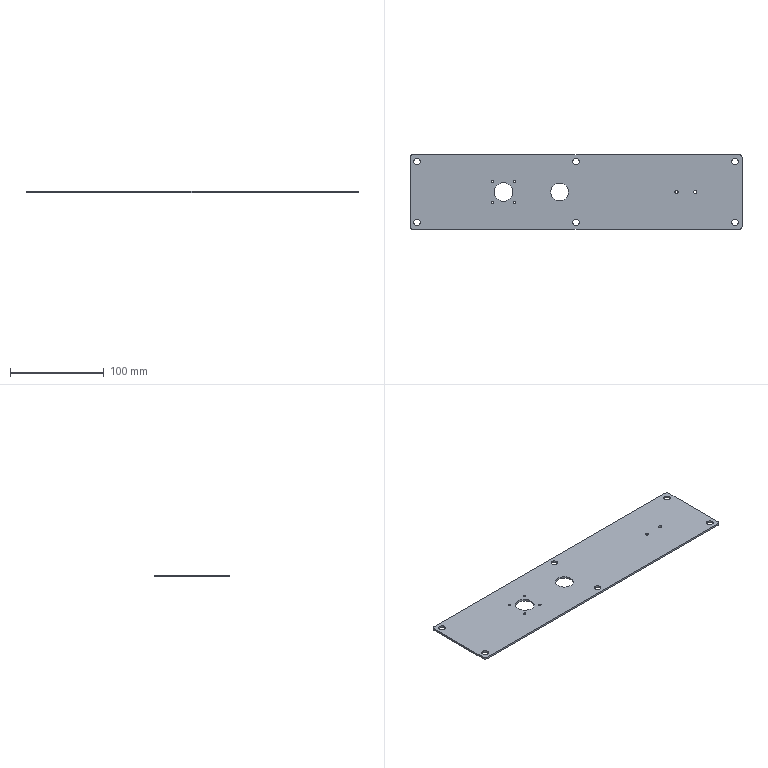Part | NX | features solid 2 | 1 solid | 38 faces | box 355 x 80 x 2 mm | volume 55052 mm3 | cylinder 32 | plane 6 | commonest cylinder face diameters 7 x12 2.459 x8 3.459 x4 6 x4 19 x2 20 x2
STEP:
#1=CARTESIAN_POINT('',(-469.229,-1630.,298.));
#2=VERTEX_POINT('',#1);
#3=CARTESIAN_POINT('',(-469.229,-1630.,300.));
#4=VERTEX_POINT('',#3);
#5=CARTESIAN_POINT('',(-469.229,-1630.,661.908));
#6=DIRECTION('',(0.,0.,-1.));
#7=VECTOR('',#6,1000.);
#8=LINE('',#5,#7);
#9=EDGE_CURVE('',#2,#4,#8,.F.);
#10=ORIENTED_EDGE('',*,*,#9,.T.);
#11=CARTESIAN_POINT('',(-465.771,-1630.,300.));
#12=VERTEX_POINT('',#11);
#13=CARTESIAN_POINT('',(-467.5,-1630.,300.));
#14=DIRECTION('',(0.,0.,1.));
#15=DIRECTION('',(-1.,0.,0.));
#16=AXIS2_PLACEMENT_3D('',#13,#14,#15);
#17=CIRCLE('',#16,1.73);
#18=EDGE_CURVE('',#4,#12,#17,.T.);
#19=ORIENTED_EDGE('',*,*,#18,.T.);
#20=CARTESIAN_POINT('',(-465.771,-1630.,298.));
#21=VERTEX_POINT('',#20);
#22=CARTESIAN_POINT('',(-465.771,-1630.,661.908));
#23=DIRECTION('',(0.,0.,-1.));
#24=VECTOR('',#23,1000.);
#25=LINE('',#22,#24);
#26=EDGE_CURVE('',#12,#21,#25,.T.);
#27=ORIENTED_EDGE('',*,*,#26,.T.);
#28=CARTESIAN_POINT('',(-467.5,-1630.,298.));
#29=DIRECTION('',(0.,0.,-1.));
#30=DIRECTION('',(1.,0.,0.));
#31=AXIS2_PLACEMENT_3D('',#28,#29,#30);
#32=CIRCLE('',#31,1.73);
#33=EDGE_CURVE('',#21,#2,#32,.T.);
#34=ORIENTED_EDGE('',*,*,#33,.T.);
#35=EDGE_LOOP('',(#10,#19,#27,#34));
#36=FACE_BOUND('',#35,.T.);
#37=CARTESIAN_POINT('',(-467.5,-1630.,661.908));
#38=DIRECTION('',(0.,0.,-1.));
#39=DIRECTION('',(1.,0.,0.));
#40=AXIS2_PLACEMENT_3D('',#37,#38,#39);
#41=CYLINDRICAL_SURFACE('',#40,1.73);
#42=ADVANCED_FACE('',(#36),#41,.F.);
#43=CARTESIAN_POINT('',(-489.229,-1630.,300.));
#44=VERTEX_POINT('',#43);
#45=CARTESIAN_POINT('',(-489.229,-1630.,298.));
#46=VERTEX_POINT('',#45);
#47=CARTESIAN_POINT('',(-489.229,-1630.,661.908));
#48=DIRECTION('',(0.,0.,-1.));
#49=VECTOR('',#48,1000.);
#50=LINE('',#47,#49);
#51=EDGE_CURVE('',#44,#46,#50,.T.);
#52=ORIENTED_EDGE('',*,*,#51,.F.);
#53=CARTESIAN_POINT('',(-485.771,-1630.,300.));
#54=VERTEX_POINT('',#53);
#55=CARTESIAN_POINT('',(-487.5,-1630.,300.));
#56=DIRECTION('',(0.,0.,1.));
#57=DIRECTION('',(-1.,0.,0.));
#58=AXIS2_PLACEMENT_3D('',#55,#56,#57);
#59=CIRCLE('',#58,1.73);
#60=EDGE_CURVE('',#44,#54,#59,.T.);
#61=ORIENTED_EDGE('',*,*,#60,.T.);
#62=CARTESIAN_POINT('',(-485.771,-1630.,298.));
#63=VERTEX_POINT('',#62);
#64=CARTESIAN_POINT('',(-485.771,-1630.,661.908));
#65=DIRECTION('',(0.,0.,-1.));
#66=VECTOR('',#65,1000.);
#67=LINE('',#64,#66);
#68=EDGE_CURVE('',#63,#54,#67,.F.);
#69=ORIENTED_EDGE('',*,*,#68,.F.);
#70=CARTESIAN_POINT('',(-487.5,-1630.,298.));
#71=DIRECTION('',(0.,0.,-1.));
#72=DIRECTION('',(1.,0.,0.));
#73=AXIS2_PLACEMENT_3D('',#70,#71,#72);
#74=CIRCLE('',#73,1.73);
#75=EDGE_CURVE('',#63,#46,#74,.T.);
#76=ORIENTED_EDGE('',*,*,#75,.T.);
#77=EDGE_LOOP('',(#52,#61,#69,#76));
#78=FACE_BOUND('',#77,.T.);
#79=CARTESIAN_POINT('',(-487.5,-1630.,661.908));
#80=DIRECTION('',(0.,0.,-1.));
#81=DIRECTION('',(1.,0.,0.));
#82=AXIS2_PLACEMENT_3D('',#79,#80,#81);
#83=CYLINDRICAL_SURFACE('',#82,1.73);
#84=ADVANCED_FACE('',(#78),#83,.F.);
#85=CARTESIAN_POINT('',(-659.78,-1641.49,300.));
#86=VERTEX_POINT('',#85);
#87=CARTESIAN_POINT('',(-659.78,-1641.49,298.));
#88=VERTEX_POINT('',#87);
#89=CARTESIAN_POINT('',(-659.78,-1641.49,-63.908));
#90=DIRECTION('',(0.,0.,1.));
#91=VECTOR('',#90,1000.);
#92=LINE('',#89,#91);
#93=EDGE_CURVE('',#86,#88,#92,.F.);
#94=ORIENTED_EDGE('',*,*,#93,.T.);
#95=CARTESIAN_POINT('',(-662.239,-1641.49,298.));
#96=VERTEX_POINT('',#95);
#97=CARTESIAN_POINT('',(-661.01,-1641.49,298.));
#98=DIRECTION('',(0.,0.,1.));
#99=DIRECTION('',(-1.,0.,0.));
#100=AXIS2_PLACEMENT_3D('',#97,#98,#99);
#101=CIRCLE('',#100,1.23);
#102=EDGE_CURVE('',#96,#88,#101,.T.);
#103=ORIENTED_EDGE('',*,*,#102,.F.);
#104=CARTESIAN_POINT('',(-662.239,-1641.49,300.));
#105=VERTEX_POINT('',#104);
#106=CARTESIAN_POINT('',(-662.239,-1641.49,-63.908));
#107=DIRECTION('',(0.,0.,1.));
#108=VECTOR('',#107,1000.);
#109=LINE('',#106,#108);
#110=EDGE_CURVE('',#96,#105,#109,.T.);
#111=ORIENTED_EDGE('',*,*,#110,.T.);
#112=CARTESIAN_POINT('',(-661.01,-1641.49,300.));
#113=DIRECTION('',(0.,0.,1.));
#114=DIRECTION('',(-1.,0.,0.));
#115=AXIS2_PLACEMENT_3D('',#112,#113,#114);
#116=CIRCLE('',#115,1.23);
#117=EDGE_CURVE('',#105,#86,#116,.T.);
#118=ORIENTED_EDGE('',*,*,#117,.T.);
#119=EDGE_LOOP('',(#94,#103,#111,#118));
#120=FACE_BOUND('',#119,.T.);
#121=CARTESIAN_POINT('',(-661.01,-1641.49,-63.908));
#122=DIRECTION('',(0.,0.,1.));
#123=DIRECTION('',(-1.,0.,0.));
#124=AXIS2_PLACEMENT_3D('',#121,#122,#123);
#125=CYLINDRICAL_SURFACE('',#124,1.23);
#126=ADVANCED_FACE('',(#120),#125,.F.);
#127=CARTESIAN_POINT('',(-659.78,-1618.51,298.));
#128=VERTEX_POINT('',#127);
#129=CARTESIAN_POINT('',(-659.78,-1618.51,300.));
#130=VERTEX_POINT('',#129);
#131=CARTESIAN_POINT('',(-659.78,-1618.51,-63.908));
#132=DIRECTION('',(0.,0.,1.));
#133=VECTOR('',#132,1000.);
#134=LINE('',#131,#133);
#135=EDGE_CURVE('',#128,#130,#134,.T.);
#136=ORIENTED_EDGE('',*,*,#135,.F.);
#137=CARTESIAN_POINT('',(-662.239,-1618.51,298.));
#138=VERTEX_POINT('',#137);
#139=CARTESIAN_POINT('',(-661.01,-1618.51,298.));
#140=DIRECTION('',(0.,0.,1.));
#141=DIRECTION('',(-1.,0.,0.));
#142=AXIS2_PLACEMENT_3D('',#139,#140,#141);
#143=CIRCLE('',#142,1.23);
#144=EDGE_CURVE('',#138,#128,#143,.T.);
#145=ORIENTED_EDGE('',*,*,#144,.F.);
#146=CARTESIAN_POINT('',(-662.239,-1618.51,300.));
#147=VERTEX_POINT('',#146);
#148=CARTESIAN_POINT('',(-662.239,-1618.51,-63.908));
#149=DIRECTION('',(0.,0.,1.));
#150=VECTOR('',#149,1000.);
#151=LINE('',#148,#150);
#152=EDGE_CURVE('',#147,#138,#151,.F.);
#153=ORIENTED_EDGE('',*,*,#152,.F.);
#154=CARTESIAN_POINT('',(-661.01,-1618.51,300.));
#155=DIRECTION('',(0.,0.,1.));
#156=DIRECTION('',(-1.,0.,0.));
#157=AXIS2_PLACEMENT_3D('',#154,#155,#156);
#158=CIRCLE('',#157,1.23);
#159=EDGE_CURVE('',#147,#130,#158,.T.);
#160=ORIENTED_EDGE('',*,*,#159,.T.);
#161=EDGE_LOOP('',(#136,#145,#153,#160));
#162=FACE_BOUND('',#161,.T.);
#163=CARTESIAN_POINT('',(-661.01,-1618.51,-63.908));
#164=DIRECTION('',(0.,0.,1.));
#165=DIRECTION('',(-1.,0.,0.));
#166=AXIS2_PLACEMENT_3D('',#163,#164,#165);
#167=CYLINDRICAL_SURFACE('',#166,1.23);
#168=ADVANCED_FACE('',(#162),#167,.F.);
#169=CARTESIAN_POINT('',(-682.761,-1618.51,300.));
#170=VERTEX_POINT('',#169);
#171=CARTESIAN_POINT('',(-682.761,-1618.51,298.));
#172=VERTEX_POINT('',#171);
#173=CARTESIAN_POINT('',(-682.761,-1618.51,-63.908));
#174=DIRECTION('',(0.,0.,1.));
#175=VECTOR('',#174,1000.);
#176=LINE('',#173,#175);
#177=EDGE_CURVE('',#170,#172,#176,.F.);
#178=ORIENTED_EDGE('',*,*,#177,.T.);
#179=CARTESIAN_POINT('',(-685.22,-1618.51,298.));
#180=VERTEX_POINT('',#179);
#181=CARTESIAN_POINT('',(-683.99,-1618.51,298.));
#182=DIRECTION('',(0.,0.,1.));
#183=DIRECTION('',(-1.,0.,0.));
#184=AXIS2_PLACEMENT_3D('',#181,#182,#183);
#185=CIRCLE('',#184,1.23);
#186=EDGE_CURVE('',#180,#172,#185,.T.);
#187=ORIENTED_EDGE('',*,*,#186,.F.);
#188=CARTESIAN_POINT('',(-685.22,-1618.51,300.));
#189=VERTEX_POINT('',#188);
#190=CARTESIAN_POINT('',(-685.22,-1618.51,-63.908));
#191=DIRECTION('',(0.,0.,1.));
#192=VECTOR('',#191,1000.);
#193=LINE('',#190,#192);
#194=EDGE_CURVE('',#180,#189,#193,.T.);
#195=ORIENTED_EDGE('',*,*,#194,.T.);
#196=CARTESIAN_POINT('',(-683.99,-1618.51,300.));
#197=DIRECTION('',(0.,0.,1.));
#198=DIRECTION('',(-1.,0.,0.));
#199=AXIS2_PLACEMENT_3D('',#196,#197,#198);
#200=CIRCLE('',#199,1.23);
#201=EDGE_CURVE('',#189,#170,#200,.T.);
#202=ORIENTED_EDGE('',*,*,#201,.T.);
#203=EDGE_LOOP('',(#178,#187,#195,#202));
#204=FACE_BOUND('',#203,.T.);
#205=CARTESIAN_POINT('',(-683.99,-1618.51,-63.908));
#206=DIRECTION('',(0.,0.,1.));
#207=DIRECTION('',(-1.,0.,0.));
#208=AXIS2_PLACEMENT_3D('',#205,#206,#207);
#209=CYLINDRICAL_SURFACE('',#208,1.23);
#210=ADVANCED_FACE('',(#204),#209,.F.);
#211=CARTESIAN_POINT('',(-682.761,-1641.49,300.));
#212=VERTEX_POINT('',#211);
#213=CARTESIAN_POINT('',(-682.761,-1641.49,298.));
#214=VERTEX_POINT('',#213);
#215=CARTESIAN_POINT('',(-682.761,-1641.49,-63.908));
#216=DIRECTION('',(0.,0.,1.));
#217=VECTOR('',#216,1000.);
#218=LINE('',#215,#217);
#219=EDGE_CURVE('',#212,#214,#218,.F.);
#220=ORIENTED_EDGE('',*,*,#219,.T.);
#221=CARTESIAN_POINT('',(-685.22,-1641.49,298.));
#222=VERTEX_POINT('',#221);
#223=CARTESIAN_POINT('',(-683.99,-1641.49,298.));
#224=DIRECTION('',(0.,0.,1.));
#225=DIRECTION('',(-1.,0.,0.));
#226=AXIS2_PLACEMENT_3D('',#223,#224,#225);
#227=CIRCLE('',#226,1.23);
#228=EDGE_CURVE('',#222,#214,#227,.T.);
#229=ORIENTED_EDGE('',*,*,#228,.F.);
#230=CARTESIAN_POINT('',(-685.22,-1641.49,300.));
#231=VERTEX_POINT('',#230);
#232=CARTESIAN_POINT('',(-685.22,-1641.49,-63.908));
#233=DIRECTION('',(0.,0.,1.));
#234=VECTOR('',#233,1000.);
#235=LINE('',#232,#234);
#236=EDGE_CURVE('',#222,#231,#235,.T.);
#237=ORIENTED_EDGE('',*,*,#236,.T.);
#238=CARTESIAN_POINT('',(-683.99,-1641.49,300.));
#239=DIRECTION('',(0.,0.,1.));
#240=DIRECTION('',(-1.,0.,0.));
#241=AXIS2_PLACEMENT_3D('',#238,#239,#240);
#242=CIRCLE('',#241,1.23);
#243=EDGE_CURVE('',#231,#212,#242,.T.);
#244=ORIENTED_EDGE('',*,*,#243,.T.);
#245=EDGE_LOOP('',(#220,#229,#237,#244));
#246=FACE_BOUND('',#245,.T.);
#247=CARTESIAN_POINT('',(-683.99,-1641.49,-63.908));
#248=DIRECTION('',(0.,0.,1.));
#249=DIRECTION('',(-1.,0.,0.));
#250=AXIS2_PLACEMENT_3D('',#247,#248,#249);
#251=CYLINDRICAL_SURFACE('',#250,1.23);
#252=ADVANCED_FACE('',(#246),#251,.F.);
#253=CARTESIAN_POINT('',(-598.5,-1662.5,298.));
#254=VERTEX_POINT('',#253);
#255=CARTESIAN_POINT('',(-598.5,-1662.5,300.));
#256=VERTEX_POINT('',#255);
#257=CARTESIAN_POINT('',(-598.5,-1662.5,298.));
#258=DIRECTION('',(0.,0.,1.));
#259=VECTOR('',#258,1000.);
#260=LINE('',#257,#259);
#261=EDGE_CURVE('',#254,#256,#260,.T.);
#262=ORIENTED_EDGE('',*,*,#261,.F.);
#263=CARTESIAN_POINT('',(-591.5,-1662.5,298.));
#264=VERTEX_POINT('',#263);
#265=CARTESIAN_POINT('',(-595.,-1662.5,298.));
#266=DIRECTION('',(0.,0.,1.));
#267=DIRECTION('',(1.,0.,0.));
#268=AXIS2_PLACEMENT_3D('',#265,#266,#267);
#269=CIRCLE('',#268,3.5);
#270=EDGE_CURVE('',#264,#254,#269,.T.);
#271=ORIENTED_EDGE('',*,*,#270,.F.);
#272=CARTESIAN_POINT('',(-591.5,-1662.5,300.));
#273=VERTEX_POINT('',#272);
#274=CARTESIAN_POINT('',(-591.5,-1662.5,298.));
#275=DIRECTION('',(0.,0.,1.));
#276=VECTOR('',#275,1000.);
#277=LINE('',#274,#276);
#278=EDGE_CURVE('',#273,#264,#277,.F.);
#279=ORIENTED_EDGE('',*,*,#278,.F.);
#280=CARTESIAN_POINT('',(-595.,-1662.5,300.));
#281=DIRECTION('',(0.,0.,-1.));
#282=DIRECTION('',(1.,0.,0.));
#283=AXIS2_PLACEMENT_3D('',#280,#281,#282);
#284=CIRCLE('',#283,3.5);
#285=EDGE_CURVE('',#256,#273,#284,.T.);
#286=ORIENTED_EDGE('',*,*,#285,.F.);
#287=EDGE_LOOP('',(#262,#271,#279,#286));
#288=FACE_BOUND('',#287,.T.);
#289=CARTESIAN_POINT('',(-595.,-1662.5,298.));
#290=DIRECTION('',(0.,0.,1.));
#291=DIRECTION('',(1.,0.,0.));
#292=AXIS2_PLACEMENT_3D('',#289,#290,#291);
#293=CYLINDRICAL_SURFACE('',#292,3.5);
#294=ADVANCED_FACE('',(#288),#293,.F.);
#295=CARTESIAN_POINT('',(-598.5,-1597.5,300.));
#296=VERTEX_POINT('',#295);
#297=CARTESIAN_POINT('',(-598.5,-1597.5,298.));
#298=VERTEX_POINT('',#297);
#299=CARTESIAN_POINT('',(-598.5,-1597.5,298.));
#300=DIRECTION('',(0.,0.,1.));
#301=VECTOR('',#300,1000.);
#302=LINE('',#299,#301);
#303=EDGE_CURVE('',#296,#298,#302,.F.);
#304=ORIENTED_EDGE('',*,*,#303,.T.);
#305=CARTESIAN_POINT('',(-591.5,-1597.5,298.));
#306=VERTEX_POINT('',#305);
#307=CARTESIAN_POINT('',(-595.,-1597.5,298.));
#308=DIRECTION('',(0.,0.,1.));
#309=DIRECTION('',(1.,0.,0.));
#310=AXIS2_PLACEMENT_3D('',#307,#308,#309);
#311=CIRCLE('',#310,3.5);
#312=EDGE_CURVE('',#306,#298,#311,.T.);
#313=ORIENTED_EDGE('',*,*,#312,.F.);
#314=CARTESIAN_POINT('',(-591.5,-1597.5,300.));
#315=VERTEX_POINT('',#314);
#316=CARTESIAN_POINT('',(-591.5,-1597.5,298.));
#317=DIRECTION('',(0.,0.,1.));
#318=VECTOR('',#317,1000.);
#319=LINE('',#316,#318);
#320=EDGE_CURVE('',#306,#315,#319,.T.);
#321=ORIENTED_EDGE('',*,*,#320,.T.);
#322=CARTESIAN_POINT('',(-595.,-1597.5,300.));
#323=DIRECTION('',(0.,0.,-1.));
#324=DIRECTION('',(1.,0.,0.));
#325=AXIS2_PLACEMENT_3D('',#322,#323,#324);
#326=CIRCLE('',#325,3.5);
#327=EDGE_CURVE('',#296,#315,#326,.T.);
#328=ORIENTED_EDGE('',*,*,#327,.F.);
#329=EDGE_LOOP('',(#304,#313,#321,#328));
#330=FACE_BOUND('',#329,.T.);
#331=CARTESIAN_POINT('',(-595.,-1597.5,298.));
#332=DIRECTION('',(0.,0.,1.));
#333=DIRECTION('',(1.,0.,0.));
#334=AXIS2_PLACEMENT_3D('',#331,#332,#333);
#335=CYLINDRICAL_SURFACE('',#334,3.5);
#336=ADVANCED_FACE('',(#330),#335,.F.);
#337=CARTESIAN_POINT('',(-768.5,-1597.5,300.));
#338=VERTEX_POINT('',#337);
#339=CARTESIAN_POINT('',(-768.5,-1597.5,298.));
#340=VERTEX_POINT('',#339);
#341=CARTESIAN_POINT('',(-768.5,-1597.5,298.));
#342=DIRECTION('',(0.,0.,1.));
#343=VECTOR('',#342,1000.);
#344=LINE('',#341,#343);
#345=EDGE_CURVE('',#338,#340,#344,.F.);
#346=ORIENTED_EDGE('',*,*,#345,.T.);
#347=CARTESIAN_POINT('',(-761.5,-1597.5,298.));
#348=VERTEX_POINT('',#347);
#349=CARTESIAN_POINT('',(-765.,-1597.5,298.));
#350=DIRECTION('',(0.,0.,1.));
#351=DIRECTION('',(1.,0.,0.));
#352=AXIS2_PLACEMENT_3D('',#349,#350,#351);
#353=CIRCLE('',#352,3.5);
#354=EDGE_CURVE('',#348,#340,#353,.T.);
#355=ORIENTED_EDGE('',*,*,#354,.F.);
#356=CARTESIAN_POINT('',(-761.5,-1597.5,300.));
#357=VERTEX_POINT('',#356);
#358=CARTESIAN_POINT('',(-761.5,-1597.5,298.));
#359=DIRECTION('',(0.,0.,1.));
#360=VECTOR('',#359,1000.);
#361=LINE('',#358,#360);
#362=EDGE_CURVE('',#348,#357,#361,.T.);
#363=ORIENTED_EDGE('',*,*,#362,.T.);
#364=CARTESIAN_POINT('',(-765.,-1597.5,300.));
#365=DIRECTION('',(0.,0.,-1.));
#366=DIRECTION('',(1.,0.,0.));
#367=AXIS2_PLACEMENT_3D('',#364,#365,#366);
#368=CIRCLE('',#367,3.5);
#369=EDGE_CURVE('',#338,#357,#368,.T.);
#370=ORIENTED_EDGE('',*,*,#369,.F.);
#371=EDGE_LOOP('',(#346,#355,#363,#370));
#372=FACE_BOUND('',#371,.T.);
#373=CARTESIAN_POINT('',(-765.,-1597.5,298.));
#374=DIRECTION('',(0.,0.,1.));
#375=DIRECTION('',(1.,0.,0.));
#376=AXIS2_PLACEMENT_3D('',#373,#374,#375);
#377=CYLINDRICAL_SURFACE('',#376,3.5);
#378=ADVANCED_FACE('',(#372),#377,.F.);
#379=CARTESIAN_POINT('',(-428.5,-1597.5,300.));
#380=VERTEX_POINT('',#379);
#381=CARTESIAN_POINT('',(-428.5,-1597.5,298.));
#382=VERTEX_POINT('',#381);
#383=CARTESIAN_POINT('',(-428.5,-1597.5,298.));
#384=DIRECTION('',(0.,0.,1.));
#385=VECTOR('',#384,1000.);
#386=LINE('',#383,#385);
#387=EDGE_CURVE('',#380,#382,#386,.F.);
#388=ORIENTED_EDGE('',*,*,#387,.T.);
#389=CARTESIAN_POINT('',(-421.5,-1597.5,298.));
#390=VERTEX_POINT('',#389);
#391=CARTESIAN_POINT('',(-425.,-1597.5,298.));
#392=DIRECTION('',(0.,0.,1.));
#393=DIRECTION('',(1.,0.,0.));
#394=AXIS2_PLACEMENT_3D('',#391,#392,#393);
#395=CIRCLE('',#394,3.5);
#396=EDGE_CURVE('',#390,#382,#395,.T.);
#397=ORIENTED_EDGE('',*,*,#396,.F.);
#398=CARTESIAN_POINT('',(-421.5,-1597.5,300.));
#399=VERTEX_POINT('',#398);
#400=CARTESIAN_POINT('',(-421.5,-1597.5,298.));
#401=DIRECTION('',(0.,0.,1.));
#402=VECTOR('',#401,1000.);
#403=LINE('',#400,#402);
#404=EDGE_CURVE('',#390,#399,#403,.T.);
#405=ORIENTED_EDGE('',*,*,#404,.T.);
#406=CARTESIAN_POINT('',(-425.,-1597.5,300.));
#407=DIRECTION('',(0.,0.,-1.));
#408=DIRECTION('',(1.,0.,0.));
#409=AXIS2_PLACEMENT_3D('',#406,#407,#408);
#410=CIRCLE('',#409,3.5);
#411=EDGE_CURVE('',#380,#399,#410,.T.);
#412=ORIENTED_EDGE('',*,*,#411,.F.);
#413=EDGE_LOOP('',(#388,#397,#405,#412));
#414=FACE_BOUND('',#413,.T.);
#415=CARTESIAN_POINT('',(-425.,-1597.5,298.));
#416=DIRECTION('',(0.,0.,1.));
#417=DIRECTION('',(1.,0.,0.));
#418=AXIS2_PLACEMENT_3D('',#415,#416,#417);
#419=CYLINDRICAL_SURFACE('',#418,3.5);
#420=ADVANCED_FACE('',(#414),#419,.F.);
#421=CARTESIAN_POINT('',(-428.5,-1662.5,300.));
#422=VERTEX_POINT('',#421);
#423=CARTESIAN_POINT('',(-428.5,-1662.5,298.));
#424=VERTEX_POINT('',#423);
#425=CARTESIAN_POINT('',(-428.5,-1662.5,298.));
#426=DIRECTION('',(0.,0.,1.));
#427=VECTOR('',#426,1000.);
#428=LINE('',#425,#427);
#429=EDGE_CURVE('',#422,#424,#428,.F.);
#430=ORIENTED_EDGE('',*,*,#429,.T.);
#431=CARTESIAN_POINT('',(-421.5,-1662.5,298.));
#432=VERTEX_POINT('',#431);
#433=CARTESIAN_POINT('',(-425.,-1662.5,298.));
#434=DIRECTION('',(0.,0.,1.));
#435=DIRECTION('',(1.,0.,0.));
#436=AXIS2_PLACEMENT_3D('',#433,#434,#435);
#437=CIRCLE('',#436,3.5);
#438=EDGE_CURVE('',#432,#424,#437,.T.);
#439=ORIENTED_EDGE('',*,*,#438,.F.);
#440=CARTESIAN_POINT('',(-421.5,-1662.5,300.));
#441=VERTEX_POINT('',#440);
#442=CARTESIAN_POINT('',(-421.5,-1662.5,298.));
#443=DIRECTION('',(0.,0.,1.));
#444=VECTOR('',#443,1000.);
#445=LINE('',#442,#444);
#446=EDGE_CURVE('',#432,#441,#445,.T.);
#447=ORIENTED_EDGE('',*,*,#446,.T.);
#448=CARTESIAN_POINT('',(-425.,-1662.5,300.));
#449=DIRECTION('',(0.,0.,-1.));
#450=DIRECTION('',(1.,0.,0.));
#451=AXIS2_PLACEMENT_3D('',#448,#449,#450);
#452=CIRCLE('',#451,3.5);
#453=EDGE_CURVE('',#422,#441,#452,.T.);
#454=ORIENTED_EDGE('',*,*,#453,.F.);
#455=EDGE_LOOP('',(#430,#439,#447,#454));
#456=FACE_BOUND('',#455,.T.);
#457=CARTESIAN_POINT('',(-425.,-1662.5,298.));
#458=DIRECTION('',(0.,0.,1.));
#459=DIRECTION('',(1.,0.,0.));
#460=AXIS2_PLACEMENT_3D('',#457,#458,#459);
#461=CYLINDRICAL_SURFACE('',#460,3.5);
#462=ADVANCED_FACE('',(#456),#461,.F.);
#463=CARTESIAN_POINT('',(-768.5,-1662.5,298.));
#464=VERTEX_POINT('',#463);
#465=CARTESIAN_POINT('',(-768.5,-1662.5,300.));
#466=VERTEX_POINT('',#465);
#467=CARTESIAN_POINT('',(-768.5,-1662.5,298.));
#468=DIRECTION('',(0.,0.,1.));
#469=VECTOR('',#468,1000.);
#470=LINE('',#467,#469);
#471=EDGE_CURVE('',#464,#466,#470,.T.);
#472=ORIENTED_EDGE('',*,*,#471,.F.);
#473=CARTESIAN_POINT('',(-761.5,-1662.5,298.));
#474=VERTEX_POINT('',#473);
#475=CARTESIAN_POINT('',(-765.,-1662.5,298.));
#476=DIRECTION('',(0.,0.,1.));
#477=DIRECTION('',(1.,0.,0.));
#478=AXIS2_PLACEMENT_3D('',#475,#476,#477);
#479=CIRCLE('',#478,3.5);
#480=EDGE_CURVE('',#474,#464,#479,.T.);
#481=ORIENTED_EDGE('',*,*,#480,.F.);
#482=CARTESIAN_POINT('',(-761.5,-1662.5,300.));
#483=VERTEX_POINT('',#482);
#484=CARTESIAN_POINT('',(-761.5,-1662.5,298.));
#485=DIRECTION('',(0.,0.,1.));
#486=VECTOR('',#485,1000.);
#487=LINE('',#484,#486);
#488=EDGE_CURVE('',#483,#474,#487,.F.);
#489=ORIENTED_EDGE('',*,*,#488,.F.);
#490=CARTESIAN_POINT('',(-765.,-1662.5,300.));
#491=DIRECTION('',(0.,0.,-1.));
#492=DIRECTION('',(1.,0.,0.));
#493=AXIS2_PLACEMENT_3D('',#490,#491,#492);
#494=CIRCLE('',#493,3.5);
#495=EDGE_CURVE('',#466,#483,#494,.T.);
#496=ORIENTED_EDGE('',*,*,#495,.F.);
#497=EDGE_LOOP('',(#472,#481,#489,#496));
#498=FACE_BOUND('',#497,.T.);
#499=CARTESIAN_POINT('',(-765.,-1662.5,298.));
#500=DIRECTION('',(0.,0.,1.));
#501=DIRECTION('',(1.,0.,0.));
#502=AXIS2_PLACEMENT_3D('',#499,#500,#501);
#503=CYLINDRICAL_SURFACE('',#502,3.5);
#504=ADVANCED_FACE('',(#498),#503,.F.);
#505=CARTESIAN_POINT('',(-417.5,-1667.,298.));
#506=VERTEX_POINT('',#505);
#507=CARTESIAN_POINT('',(-420.5,-1670.,298.));
#508=VERTEX_POINT('',#507);
#509=CARTESIAN_POINT('',(-420.5,-1667.,298.));
#510=DIRECTION('',(0.,0.,-1.));
#511=DIRECTION('',(-1.,0.,0.));
#512=AXIS2_PLACEMENT_3D('',#509,#510,#511);
#513=CIRCLE('',#512,3.);
#514=EDGE_CURVE('',#506,#508,#513,.T.);
#515=ORIENTED_EDGE('',*,*,#514,.F.);
#516=CARTESIAN_POINT('',(-417.5,-1667.,300.));
#517=VERTEX_POINT('',#516);
#518=CARTESIAN_POINT('',(-417.5,-1667.,298.));
#519=DIRECTION('',(0.,0.,-1.));
#520=VECTOR('',#519,1000.);
#521=LINE('',#518,#520);
#522=EDGE_CURVE('',#517,#506,#521,.T.);
#523=ORIENTED_EDGE('',*,*,#522,.F.);
#524=CARTESIAN_POINT('',(-420.5,-1670.,300.));
#525=VERTEX_POINT('',#524);
#526=CARTESIAN_POINT('',(-420.5,-1667.,300.));
#527=DIRECTION('',(0.,0.,1.));
#528=DIRECTION('',(-1.,0.,0.));
#529=AXIS2_PLACEMENT_3D('',#526,#527,#528);
#530=CIRCLE('',#529,3.);
#531=EDGE_CURVE('',#525,#517,#530,.T.);
#532=ORIENTED_EDGE('',*,*,#531,.F.);
#533=CARTESIAN_POINT('',(-420.5,-1670.,298.));
#534=DIRECTION('',(0.,0.,1.));
#535=VECTOR('',#534,1000.);
#536=LINE('',#533,#535);
#537=EDGE_CURVE('',#508,#525,#536,.T.);
#538=ORIENTED_EDGE('',*,*,#537,.F.);
#539=EDGE_LOOP('',(#515,#523,#532,#538));
#540=FACE_BOUND('',#539,.T.);
#541=CARTESIAN_POINT('',(-420.5,-1667.,298.));
#542=DIRECTION('',(0.,0.,1.));
#543=DIRECTION('',(0.,1.,0.));
#544=AXIS2_PLACEMENT_3D('',#541,#542,#543);
#545=CYLINDRICAL_SURFACE('',#544,3.);
#546=ADVANCED_FACE('',(#540),#545,.T.);
#547=CARTESIAN_POINT('',(-769.5,-1670.,298.));
#548=VERTEX_POINT('',#547);
#549=CARTESIAN_POINT('',(-772.5,-1667.,298.));
#550=VERTEX_POINT('',#549);
#551=CARTESIAN_POINT('',(-769.5,-1667.,298.));
#552=DIRECTION('',(0.,0.,-1.));
#553=DIRECTION('',(-1.,0.,0.));
#554=AXIS2_PLACEMENT_3D('',#551,#552,#553);
#555=CIRCLE('',#554,3.);
#556=EDGE_CURVE('',#548,#550,#555,.T.);
#557=ORIENTED_EDGE('',*,*,#556,.F.);
#558=CARTESIAN_POINT('',(-769.5,-1670.,300.));
#559=VERTEX_POINT('',#558);
#560=CARTESIAN_POINT('',(-769.5,-1670.,298.));
#561=DIRECTION('',(0.,0.,-1.));
#562=VECTOR('',#561,1000.);
#563=LINE('',#560,#562);
#564=EDGE_CURVE('',#559,#548,#563,.T.);
#565=ORIENTED_EDGE('',*,*,#564,.F.);
#566=CARTESIAN_POINT('',(-772.5,-1667.,300.));
#567=VERTEX_POINT('',#566);
#568=CARTESIAN_POINT('',(-769.5,-1667.,300.));
#569=DIRECTION('',(0.,0.,1.));
#570=DIRECTION('',(-1.,0.,0.));
#571=AXIS2_PLACEMENT_3D('',#568,#569,#570);
#572=CIRCLE('',#571,3.);
#573=EDGE_CURVE('',#567,#559,#572,.T.);
#574=ORIENTED_EDGE('',*,*,#573,.F.);
#575=CARTESIAN_POINT('',(-772.5,-1667.,298.));
#576=DIRECTION('',(0.,0.,1.));
#577=VECTOR('',#576,1000.);
#578=LINE('',#575,#577);
#579=EDGE_CURVE('',#550,#567,#578,.T.);
#580=ORIENTED_EDGE('',*,*,#579,.F.);
#581=EDGE_LOOP('',(#557,#565,#574,#580));
#582=FACE_BOUND('',#581,.T.);
#583=CARTESIAN_POINT('',(-769.5,-1667.,298.));
#584=DIRECTION('',(0.,0.,1.));
#585=DIRECTION('',(0.,1.,0.));
#586=AXIS2_PLACEMENT_3D('',#583,#584,#585);
#587=CYLINDRICAL_SURFACE('',#586,3.);
#588=ADVANCED_FACE('',(#582),#587,.T.);
#589=CARTESIAN_POINT('',(-420.5,-1590.,298.));
#590=VERTEX_POINT('',#589);
#591=CARTESIAN_POINT('',(-417.5,-1593.,298.));
#592=VERTEX_POINT('',#591);
#593=CARTESIAN_POINT('',(-420.5,-1593.,298.));
#594=DIRECTION('',(0.,0.,-1.));
#595=DIRECTION('',(-1.,0.,0.));
#596=AXIS2_PLACEMENT_3D('',#593,#594,#595);
#597=CIRCLE('',#596,3.);
#598=EDGE_CURVE('',#590,#592,#597,.T.);
#599=ORIENTED_EDGE('',*,*,#598,.F.);
#600=CARTESIAN_POINT('',(-420.5,-1590.,300.));
#601=VERTEX_POINT('',#600);
#602=CARTESIAN_POINT('',(-420.5,-1590.,298.));
#603=DIRECTION('',(0.,0.,-1.));
#604=VECTOR('',#603,1000.);
#605=LINE('',#602,#604);
#606=EDGE_CURVE('',#601,#590,#605,.T.);
#607=ORIENTED_EDGE('',*,*,#606,.F.);
#608=CARTESIAN_POINT('',(-417.5,-1593.,300.));
#609=VERTEX_POINT('',#608);
#610=CARTESIAN_POINT('',(-420.5,-1593.,300.));
#611=DIRECTION('',(0.,0.,1.));
#612=DIRECTION('',(-1.,0.,0.));
#613=AXIS2_PLACEMENT_3D('',#610,#611,#612);
#614=CIRCLE('',#613,3.);
#615=EDGE_CURVE('',#609,#601,#614,.T.);
#616=ORIENTED_EDGE('',*,*,#615,.F.);
#617=CARTESIAN_POINT('',(-417.5,-1593.,298.));
#618=DIRECTION('',(0.,0.,1.));
#619=VECTOR('',#618,1000.);
#620=LINE('',#617,#619);
#621=EDGE_CURVE('',#592,#609,#620,.T.);
#622=ORIENTED_EDGE('',*,*,#621,.F.);
#623=EDGE_LOOP('',(#599,#607,#616,#622));
#624=FACE_BOUND('',#623,.T.);
#625=CARTESIAN_POINT('',(-420.5,-1593.,298.));
#626=DIRECTION('',(0.,0.,1.));
#627=DIRECTION('',(0.,1.,0.));
#628=AXIS2_PLACEMENT_3D('',#625,#626,#627);
#629=CYLINDRICAL_SURFACE('',#628,3.);
#630=ADVANCED_FACE('',(#624),#629,.T.);
#631=CARTESIAN_POINT('',(-772.5,-1593.,298.));
#632=VERTEX_POINT('',#631);
#633=CARTESIAN_POINT('',(-769.5,-1590.,298.));
#634=VERTEX_POINT('',#633);
#635=CARTESIAN_POINT('',(-769.5,-1593.,298.));
#636=DIRECTION('',(0.,0.,-1.));
#637=DIRECTION('',(-1.,0.,0.));
#638=AXIS2_PLACEMENT_3D('',#635,#636,#637);
#639=CIRCLE('',#638,3.);
#640=EDGE_CURVE('',#632,#634,#639,.T.);
#641=ORIENTED_EDGE('',*,*,#640,.F.);
#642=CARTESIAN_POINT('',(-772.5,-1593.,300.));
#643=VERTEX_POINT('',#642);
#644=CARTESIAN_POINT('',(-772.5,-1593.,298.));
#645=DIRECTION('',(0.,0.,-1.));
#646=VECTOR('',#645,1000.);
#647=LINE('',#644,#646);
#648=EDGE_CURVE('',#643,#632,#647,.T.);
#649=ORIENTED_EDGE('',*,*,#648,.F.);
#650=CARTESIAN_POINT('',(-769.5,-1590.,300.));
#651=VERTEX_POINT('',#650);
#652=CARTESIAN_POINT('',(-769.5,-1593.,300.));
#653=DIRECTION('',(0.,0.,1.));
#654=DIRECTION('',(-1.,0.,0.));
#655=AXIS2_PLACEMENT_3D('',#652,#653,#654);
#656=CIRCLE('',#655,3.);
#657=EDGE_CURVE('',#651,#643,#656,.T.);
#658=ORIENTED_EDGE('',*,*,#657,.F.);
#659=CARTESIAN_POINT('',(-769.5,-1590.,298.));
#660=DIRECTION('',(0.,0.,1.));
#661=VECTOR('',#660,1000.);
#662=LINE('',#659,#661);
#663=EDGE_CURVE('',#634,#651,#662,.T.);
#664=ORIENTED_EDGE('',*,*,#663,.F.);
#665=EDGE_LOOP('',(#641,#649,#658,#664));
#666=FACE_BOUND('',#665,.T.);
#667=CARTESIAN_POINT('',(-769.5,-1593.,298.));
#668=DIRECTION('',(0.,0.,1.));
#669=DIRECTION('',(0.,1.,0.));
#670=AXIS2_PLACEMENT_3D('',#667,#668,#669);
#671=CYLINDRICAL_SURFACE('',#670,3.);
#672=ADVANCED_FACE('',(#666),#671,.T.);
#673=CARTESIAN_POINT('',(-603.,-1630.,298.));
#674=VERTEX_POINT('',#673);
#675=CARTESIAN_POINT('',(-603.,-1630.,300.));
#676=VERTEX_POINT('',#675);
#677=CARTESIAN_POINT('',(-603.,-1630.,-63.908));
#678=DIRECTION('',(0.,0.,1.));
#679=VECTOR('',#678,1000.);
#680=LINE('',#677,#679);
#681=EDGE_CURVE('',#674,#676,#680,.T.);
#682=ORIENTED_EDGE('',*,*,#681,.F.);
#683=CARTESIAN_POINT('',(-622.,-1630.,298.));
#684=VERTEX_POINT('',#683);
#685=CARTESIAN_POINT('',(-612.5,-1630.,298.));
#686=DIRECTION('',(0.,0.,1.));
#687=DIRECTION('',(-1.,0.,0.));
#688=AXIS2_PLACEMENT_3D('',#685,#686,#687);
#689=CIRCLE('',#688,9.5);
#690=EDGE_CURVE('',#684,#674,#689,.T.);
#691=ORIENTED_EDGE('',*,*,#690,.F.);
#692=CARTESIAN_POINT('',(-622.,-1630.,300.));
#693=VERTEX_POINT('',#692);
#694=CARTESIAN_POINT('',(-622.,-1630.,-63.908));
#695=DIRECTION('',(0.,0.,1.));
#696=VECTOR('',#695,1000.);
#697=LINE('',#694,#696);
#698=EDGE_CURVE('',#693,#684,#697,.F.);
#699=ORIENTED_EDGE('',*,*,#698,.F.);
#700=CARTESIAN_POINT('',(-612.5,-1630.,300.));
#701=DIRECTION('',(0.,0.,1.));
#702=DIRECTION('',(-1.,0.,0.));
#703=AXIS2_PLACEMENT_3D('',#700,#701,#702);
#704=CIRCLE('',#703,9.5);
#705=EDGE_CURVE('',#693,#676,#704,.T.);
#706=ORIENTED_EDGE('',*,*,#705,.T.);
#707=EDGE_LOOP('',(#682,#691,#699,#706));
#708=FACE_BOUND('',#707,.T.);
#709=CARTESIAN_POINT('',(-612.5,-1630.,-63.908));
#710=DIRECTION('',(0.,0.,1.));
#711=DIRECTION('',(-1.,0.,0.));
#712=AXIS2_PLACEMENT_3D('',#709,#710,#711);
#713=CYLINDRICAL_SURFACE('',#712,9.5);
#714=ADVANCED_FACE('',(#708),#713,.F.);
#715=CARTESIAN_POINT('',(-662.5,-1630.,298.));
#716=VERTEX_POINT('',#715);
#717=CARTESIAN_POINT('',(-662.5,-1630.,300.));
#718=VERTEX_POINT('',#717);
#719=CARTESIAN_POINT('',(-662.5,-1630.,-63.908));
#720=DIRECTION('',(0.,0.,1.));
#721=VECTOR('',#720,1000.);
#722=LINE('',#719,#721);
#723=EDGE_CURVE('',#716,#718,#722,.T.);
#724=ORIENTED_EDGE('',*,*,#723,.F.);
#725=CARTESIAN_POINT('',(-682.5,-1630.,298.));
#726=VERTEX_POINT('',#725);
#727=CARTESIAN_POINT('',(-672.5,-1630.,298.));
#728=DIRECTION('',(0.,0.,1.));
#729=DIRECTION('',(-1.,0.,0.));
#730=AXIS2_PLACEMENT_3D('',#727,#728,#729);
#731=CIRCLE('',#730,10.);
#732=EDGE_CURVE('',#726,#716,#731,.T.);
#733=ORIENTED_EDGE('',*,*,#732,.F.);
#734=CARTESIAN_POINT('',(-682.5,-1630.,300.));
#735=VERTEX_POINT('',#734);
#736=CARTESIAN_POINT('',(-682.5,-1630.,-63.908));
#737=DIRECTION('',(0.,0.,1.));
#738=VECTOR('',#737,1000.);
#739=LINE('',#736,#738);
#740=EDGE_CURVE('',#735,#726,#739,.F.);
#741=ORIENTED_EDGE('',*,*,#740,.F.);
#742=CARTESIAN_POINT('',(-672.5,-1630.,300.));
#743=DIRECTION('',(0.,0.,1.));
#744=DIRECTION('',(-1.,0.,0.));
#745=AXIS2_PLACEMENT_3D('',#742,#743,#744);
#746=CIRCLE('',#745,10.);
#747=EDGE_CURVE('',#735,#718,#746,.T.);
#748=ORIENTED_EDGE('',*,*,#747,.T.);
#749=EDGE_LOOP('',(#724,#733,#741,#748));
#750=FACE_BOUND('',#749,.T.);
#751=CARTESIAN_POINT('',(-672.5,-1630.,-63.908));
#752=DIRECTION('',(0.,0.,1.));
#753=DIRECTION('',(-1.,0.,0.));
#754=AXIS2_PLACEMENT_3D('',#751,#752,#753);
#755=CYLINDRICAL_SURFACE('',#754,10.);
#756=ADVANCED_FACE('',(#750),#755,.F.);
#757=ORIENTED_EDGE('',*,*,#747,.F.);
#758=CARTESIAN_POINT('',(-672.5,-1630.,300.));
#759=DIRECTION('',(0.,0.,1.));
#760=DIRECTION('',(-1.,0.,0.));
#761=AXIS2_PLACEMENT_3D('',#758,#759,#760);
#762=CIRCLE('',#761,10.);
#763=EDGE_CURVE('',#718,#735,#762,.T.);
#764=ORIENTED_EDGE('',*,*,#763,.F.);
#765=EDGE_LOOP('',(#757,#764));
#766=FACE_BOUND('',#765,.T.);
#767=ORIENTED_EDGE('',*,*,#705,.F.);
#768=CARTESIAN_POINT('',(-612.5,-1630.,300.));
#769=DIRECTION('',(0.,0.,1.));
#770=DIRECTION('',(-1.,0.,0.));
#771=AXIS2_PLACEMENT_3D('',#768,#769,#770);
#772=CIRCLE('',#771,9.5);
#773=EDGE_CURVE('',#676,#693,#772,.T.);
#774=ORIENTED_EDGE('',*,*,#773,.F.);
#775=EDGE_LOOP('',(#767,#774));
#776=FACE_BOUND('',#775,.T.);
#777=CARTESIAN_POINT('',(-765.,-1662.5,300.));
#778=DIRECTION('',(0.,0.,-1.));
#779=DIRECTION('',(1.,0.,0.));
#780=AXIS2_PLACEMENT_3D('',#777,#778,#779);
#781=CIRCLE('',#780,3.5);
#782=EDGE_CURVE('',#483,#466,#781,.T.);
#783=ORIENTED_EDGE('',*,*,#782,.T.);
#784=ORIENTED_EDGE('',*,*,#495,.T.);
#785=EDGE_LOOP('',(#783,#784));
#786=FACE_BOUND('',#785,.T.);
#787=CARTESIAN_POINT('',(-425.,-1662.5,300.));
#788=DIRECTION('',(0.,0.,-1.));
#789=DIRECTION('',(1.,0.,0.));
#790=AXIS2_PLACEMENT_3D('',#787,#788,#789);
#791=CIRCLE('',#790,3.5);
#792=EDGE_CURVE('',#441,#422,#791,.T.);
#793=ORIENTED_EDGE('',*,*,#792,.T.);
#794=ORIENTED_EDGE('',*,*,#453,.T.);
#795=EDGE_LOOP('',(#793,#794));
#796=FACE_BOUND('',#795,.T.);
#797=CARTESIAN_POINT('',(-425.,-1597.5,300.));
#798=DIRECTION('',(0.,0.,-1.));
#799=DIRECTION('',(1.,0.,0.));
#800=AXIS2_PLACEMENT_3D('',#797,#798,#799);
#801=CIRCLE('',#800,3.5);
#802=EDGE_CURVE('',#399,#380,#801,.T.);
#803=ORIENTED_EDGE('',*,*,#802,.T.);
#804=ORIENTED_EDGE('',*,*,#411,.T.);
#805=EDGE_LOOP('',(#803,#804));
#806=FACE_BOUND('',#805,.T.);
#807=CARTESIAN_POINT('',(-765.,-1597.5,300.));
#808=DIRECTION('',(0.,0.,-1.));
#809=DIRECTION('',(1.,0.,0.));
#810=AXIS2_PLACEMENT_3D('',#807,#808,#809);
#811=CIRCLE('',#810,3.5);
#812=EDGE_CURVE('',#357,#338,#811,.T.);
#813=ORIENTED_EDGE('',*,*,#812,.T.);
#814=ORIENTED_EDGE('',*,*,#369,.T.);
#815=EDGE_LOOP('',(#813,#814));
#816=FACE_BOUND('',#815,.T.);
#817=CARTESIAN_POINT('',(-595.,-1597.5,300.));
#818=DIRECTION('',(0.,0.,-1.));
#819=DIRECTION('',(1.,0.,0.));
#820=AXIS2_PLACEMENT_3D('',#817,#818,#819);
#821=CIRCLE('',#820,3.5);
#822=EDGE_CURVE('',#315,#296,#821,.T.);
#823=ORIENTED_EDGE('',*,*,#822,.T.);
#824=ORIENTED_EDGE('',*,*,#327,.T.);
#825=EDGE_LOOP('',(#823,#824));
#826=FACE_BOUND('',#825,.T.);
#827=CARTESIAN_POINT('',(-595.,-1662.5,300.));
#828=DIRECTION('',(0.,0.,-1.));
#829=DIRECTION('',(1.,0.,0.));
#830=AXIS2_PLACEMENT_3D('',#827,#828,#829);
#831=CIRCLE('',#830,3.5);
#832=EDGE_CURVE('',#273,#256,#831,.T.);
#833=ORIENTED_EDGE('',*,*,#832,.T.);
#834=ORIENTED_EDGE('',*,*,#285,.T.);
#835=EDGE_LOOP('',(#833,#834));
#836=FACE_BOUND('',#835,.T.);
#837=ORIENTED_EDGE('',*,*,#243,.F.);
#838=CARTESIAN_POINT('',(-683.99,-1641.49,300.));
#839=DIRECTION('',(0.,0.,1.));
#840=DIRECTION('',(-1.,0.,0.));
#841=AXIS2_PLACEMENT_3D('',#838,#839,#840);
#842=CIRCLE('',#841,1.23);
#843=EDGE_CURVE('',#212,#231,#842,.T.);
#844=ORIENTED_EDGE('',*,*,#843,.F.);
#845=EDGE_LOOP('',(#837,#844));
#846=FACE_BOUND('',#845,.T.);
#847=ORIENTED_EDGE('',*,*,#201,.F.);
#848=CARTESIAN_POINT('',(-683.99,-1618.51,300.));
#849=DIRECTION('',(0.,0.,1.));
#850=DIRECTION('',(-1.,0.,0.));
#851=AXIS2_PLACEMENT_3D('',#848,#849,#850);
#852=CIRCLE('',#851,1.23);
#853=EDGE_CURVE('',#170,#189,#852,.T.);
#854=ORIENTED_EDGE('',*,*,#853,.F.);
#855=EDGE_LOOP('',(#847,#854));
#856=FACE_BOUND('',#855,.T.);
#857=ORIENTED_EDGE('',*,*,#159,.F.);
#858=CARTESIAN_POINT('',(-661.01,-1618.51,300.));
#859=DIRECTION('',(0.,0.,1.));
#860=DIRECTION('',(-1.,0.,0.));
#861=AXIS2_PLACEMENT_3D('',#858,#859,#860);
#862=CIRCLE('',#861,1.23);
#863=EDGE_CURVE('',#130,#147,#862,.T.);
#864=ORIENTED_EDGE('',*,*,#863,.F.);
#865=EDGE_LOOP('',(#857,#864));
#866=FACE_BOUND('',#865,.T.);
#867=ORIENTED_EDGE('',*,*,#117,.F.);
#868=CARTESIAN_POINT('',(-661.01,-1641.49,300.));
#869=DIRECTION('',(0.,0.,1.));
#870=DIRECTION('',(-1.,0.,0.));
#871=AXIS2_PLACEMENT_3D('',#868,#869,#870);
#872=CIRCLE('',#871,1.23);
#873=EDGE_CURVE('',#86,#105,#872,.T.);
#874=ORIENTED_EDGE('',*,*,#873,.F.);
#875=EDGE_LOOP('',(#867,#874));
#876=FACE_BOUND('',#875,.T.);
#877=CARTESIAN_POINT('',(-487.5,-1630.,300.));
#878=DIRECTION('',(0.,0.,1.));
#879=DIRECTION('',(-1.,0.,0.));
#880=AXIS2_PLACEMENT_3D('',#877,#878,#879);
#881=CIRCLE('',#880,1.73);
#882=EDGE_CURVE('',#54,#44,#881,.T.);
#883=ORIENTED_EDGE('',*,*,#882,.F.);
#884=ORIENTED_EDGE('',*,*,#60,.F.);
#885=EDGE_LOOP('',(#883,#884));
#886=FACE_BOUND('',#885,.T.);
#887=CARTESIAN_POINT('',(-467.5,-1630.,300.));
#888=DIRECTION('',(0.,0.,1.));
#889=DIRECTION('',(-1.,0.,0.));
#890=AXIS2_PLACEMENT_3D('',#887,#888,#889);
#891=CIRCLE('',#890,1.73);
#892=EDGE_CURVE('',#12,#4,#891,.T.);
#893=ORIENTED_EDGE('',*,*,#892,.F.);
#894=ORIENTED_EDGE('',*,*,#18,.F.);
#895=EDGE_LOOP('',(#893,#894));
#896=FACE_BOUND('',#895,.T.);
#897=CARTESIAN_POINT('',(-417.5,-1590.,300.));
#898=DIRECTION('',(-1.,0.,0.));
#899=VECTOR('',#898,1000.);
#900=LINE('',#897,#899);
#901=EDGE_CURVE('',#601,#651,#900,.T.);
#902=ORIENTED_EDGE('',*,*,#901,.T.);
#903=ORIENTED_EDGE('',*,*,#657,.T.);
#904=CARTESIAN_POINT('',(-772.5,-1590.,300.));
#905=DIRECTION('',(0.,-1.,0.));
#906=VECTOR('',#905,1000.);
#907=LINE('',#904,#906);
#908=EDGE_CURVE('',#643,#567,#907,.T.);
#909=ORIENTED_EDGE('',*,*,#908,.T.);
#910=ORIENTED_EDGE('',*,*,#573,.T.);
#911=CARTESIAN_POINT('',(-772.5,-1670.,300.));
#912=DIRECTION('',(1.,0.,0.));
#913=VECTOR('',#912,1000.);
#914=LINE('',#911,#913);
#915=EDGE_CURVE('',#559,#525,#914,.T.);
#916=ORIENTED_EDGE('',*,*,#915,.T.);
#917=ORIENTED_EDGE('',*,*,#531,.T.);
#918=CARTESIAN_POINT('',(-417.5,-1670.,300.));
#919=DIRECTION('',(0.,1.,0.));
#920=VECTOR('',#919,1000.);
#921=LINE('',#918,#920);
#922=EDGE_CURVE('',#517,#609,#921,.T.);
#923=ORIENTED_EDGE('',*,*,#922,.T.);
#924=ORIENTED_EDGE('',*,*,#615,.T.);
#925=EDGE_LOOP('',(#902,#903,#909,#910,#916,#917,#923,#924));
#926=FACE_BOUND('',#925,.T.);
#927=CARTESIAN_POINT('',(-417.5,-1590.,300.));
#928=DIRECTION('',(0.,0.,1.));
#929=DIRECTION('',(0.,-1.,0.));
#930=AXIS2_PLACEMENT_3D('',#927,#928,#929);
#931=PLANE('',#930);
#932=ADVANCED_FACE('',(#766,#776,#786,#796,#806,#816,#826,#836,#846,#856,#866,#876,#886,#896,#926),#931,.T.);
#933=ORIENTED_EDGE('',*,*,#732,.T.);
#934=CARTESIAN_POINT('',(-672.5,-1630.,298.));
#935=DIRECTION('',(0.,0.,1.));
#936=DIRECTION('',(-1.,0.,0.));
#937=AXIS2_PLACEMENT_3D('',#934,#935,#936);
#938=CIRCLE('',#937,10.);
#939=EDGE_CURVE('',#716,#726,#938,.T.);
#940=ORIENTED_EDGE('',*,*,#939,.T.);
#941=EDGE_LOOP('',(#933,#940));
#942=FACE_BOUND('',#941,.T.);
#943=ORIENTED_EDGE('',*,*,#690,.T.);
#944=CARTESIAN_POINT('',(-612.5,-1630.,298.));
#945=DIRECTION('',(0.,0.,1.));
#946=DIRECTION('',(-1.,0.,0.));
#947=AXIS2_PLACEMENT_3D('',#944,#945,#946);
#948=CIRCLE('',#947,9.5);
#949=EDGE_CURVE('',#674,#684,#948,.T.);
#950=ORIENTED_EDGE('',*,*,#949,.T.);
#951=EDGE_LOOP('',(#943,#950));
#952=FACE_BOUND('',#951,.T.);
#953=ORIENTED_EDGE('',*,*,#480,.T.);
#954=CARTESIAN_POINT('',(-765.,-1662.5,298.));
#955=DIRECTION('',(0.,0.,1.));
#956=DIRECTION('',(1.,0.,0.));
#957=AXIS2_PLACEMENT_3D('',#954,#955,#956);
#958=CIRCLE('',#957,3.5);
#959=EDGE_CURVE('',#464,#474,#958,.T.);
#960=ORIENTED_EDGE('',*,*,#959,.T.);
#961=EDGE_LOOP('',(#953,#960));
#962=FACE_BOUND('',#961,.T.);
#963=ORIENTED_EDGE('',*,*,#438,.T.);
#964=CARTESIAN_POINT('',(-425.,-1662.5,298.));
#965=DIRECTION('',(0.,0.,1.));
#966=DIRECTION('',(1.,0.,0.));
#967=AXIS2_PLACEMENT_3D('',#964,#965,#966);
#968=CIRCLE('',#967,3.5);
#969=EDGE_CURVE('',#424,#432,#968,.T.);
#970=ORIENTED_EDGE('',*,*,#969,.T.);
#971=EDGE_LOOP('',(#963,#970));
#972=FACE_BOUND('',#971,.T.);
#973=ORIENTED_EDGE('',*,*,#396,.T.);
#974=CARTESIAN_POINT('',(-425.,-1597.5,298.));
#975=DIRECTION('',(0.,0.,1.));
#976=DIRECTION('',(1.,0.,0.));
#977=AXIS2_PLACEMENT_3D('',#974,#975,#976);
#978=CIRCLE('',#977,3.5);
#979=EDGE_CURVE('',#382,#390,#978,.T.);
#980=ORIENTED_EDGE('',*,*,#979,.T.);
#981=EDGE_LOOP('',(#973,#980));
#982=FACE_BOUND('',#981,.T.);
#983=ORIENTED_EDGE('',*,*,#354,.T.);
#984=CARTESIAN_POINT('',(-765.,-1597.5,298.));
#985=DIRECTION('',(0.,0.,1.));
#986=DIRECTION('',(1.,0.,0.));
#987=AXIS2_PLACEMENT_3D('',#984,#985,#986);
#988=CIRCLE('',#987,3.5);
#989=EDGE_CURVE('',#340,#348,#988,.T.);
#990=ORIENTED_EDGE('',*,*,#989,.T.);
#991=EDGE_LOOP('',(#983,#990));
#992=FACE_BOUND('',#991,.T.);
#993=ORIENTED_EDGE('',*,*,#312,.T.);
#994=CARTESIAN_POINT('',(-595.,-1597.5,298.));
#995=DIRECTION('',(0.,0.,1.));
#996=DIRECTION('',(1.,0.,0.));
#997=AXIS2_PLACEMENT_3D('',#994,#995,#996);
#998=CIRCLE('',#997,3.5);
#999=EDGE_CURVE('',#298,#306,#998,.T.);
#1000=ORIENTED_EDGE('',*,*,#999,.T.);
#1001=EDGE_LOOP('',(#993,#1000));
#1002=FACE_BOUND('',#1001,.T.);
#1003=ORIENTED_EDGE('',*,*,#270,.T.);
#1004=CARTESIAN_POINT('',(-595.,-1662.5,298.));
#1005=DIRECTION('',(0.,0.,1.));
#1006=DIRECTION('',(1.,0.,0.));
#1007=AXIS2_PLACEMENT_3D('',#1004,#1005,#1006);
#1008=CIRCLE('',#1007,3.5);
#1009=EDGE_CURVE('',#254,#264,#1008,.T.);
#1010=ORIENTED_EDGE('',*,*,#1009,.T.);
#1011=EDGE_LOOP('',(#1003,#1010));
#1012=FACE_BOUND('',#1011,.T.);
#1013=ORIENTED_EDGE('',*,*,#228,.T.);
#1014=CARTESIAN_POINT('',(-683.99,-1641.49,298.));
#1015=DIRECTION('',(0.,0.,1.));
#1016=DIRECTION('',(-1.,0.,0.));
#1017=AXIS2_PLACEMENT_3D('',#1014,#1015,#1016);
#1018=CIRCLE('',#1017,1.23);
#1019=EDGE_CURVE('',#214,#222,#1018,.T.);
#1020=ORIENTED_EDGE('',*,*,#1019,.T.);
#1021=EDGE_LOOP('',(#1013,#1020));
#1022=FACE_BOUND('',#1021,.T.);
#1023=ORIENTED_EDGE('',*,*,#186,.T.);
#1024=CARTESIAN_POINT('',(-683.99,-1618.51,298.));
#1025=DIRECTION('',(0.,0.,1.));
#1026=DIRECTION('',(-1.,0.,0.));
#1027=AXIS2_PLACEMENT_3D('',#1024,#1025,#1026);
#1028=CIRCLE('',#1027,1.23);
#1029=EDGE_CURVE('',#172,#180,#1028,.T.);
#1030=ORIENTED_EDGE('',*,*,#1029,.T.);
#1031=EDGE_LOOP('',(#1023,#1030));
#1032=FACE_BOUND('',#1031,.T.);
#1033=ORIENTED_EDGE('',*,*,#144,.T.);
#1034=CARTESIAN_POINT('',(-661.01,-1618.51,298.));
#1035=DIRECTION('',(0.,0.,1.));
#1036=DIRECTION('',(-1.,0.,0.));
#1037=AXIS2_PLACEMENT_3D('',#1034,#1035,#1036);
#1038=CIRCLE('',#1037,1.23);
#1039=EDGE_CURVE('',#128,#138,#1038,.T.);
#1040=ORIENTED_EDGE('',*,*,#1039,.T.);
#1041=EDGE_LOOP('',(#1033,#1040));
#1042=FACE_BOUND('',#1041,.T.);
#1043=ORIENTED_EDGE('',*,*,#102,.T.);
#1044=CARTESIAN_POINT('',(-661.01,-1641.49,298.));
#1045=DIRECTION('',(0.,0.,1.));
#1046=DIRECTION('',(-1.,0.,0.));
#1047=AXIS2_PLACEMENT_3D('',#1044,#1045,#1046);
#1048=CIRCLE('',#1047,1.23);
#1049=EDGE_CURVE('',#88,#96,#1048,.T.);
#1050=ORIENTED_EDGE('',*,*,#1049,.T.);
#1051=EDGE_LOOP('',(#1043,#1050));
#1052=FACE_BOUND('',#1051,.T.);
#1053=ORIENTED_EDGE('',*,*,#75,.F.);
#1054=CARTESIAN_POINT('',(-487.5,-1630.,298.));
#1055=DIRECTION('',(0.,0.,-1.));
#1056=DIRECTION('',(1.,0.,0.));
#1057=AXIS2_PLACEMENT_3D('',#1054,#1055,#1056);
#1058=CIRCLE('',#1057,1.73);
#1059=EDGE_CURVE('',#46,#63,#1058,.T.);
#1060=ORIENTED_EDGE('',*,*,#1059,.F.);
#1061=EDGE_LOOP('',(#1053,#1060));
#1062=FACE_BOUND('',#1061,.T.);
#1063=ORIENTED_EDGE('',*,*,#33,.F.);
#1064=CARTESIAN_POINT('',(-467.5,-1630.,298.));
#1065=DIRECTION('',(0.,0.,-1.));
#1066=DIRECTION('',(1.,0.,0.));
#1067=AXIS2_PLACEMENT_3D('',#1064,#1065,#1066);
#1068=CIRCLE('',#1067,1.73);
#1069=EDGE_CURVE('',#2,#21,#1068,.T.);
#1070=ORIENTED_EDGE('',*,*,#1069,.F.);
#1071=EDGE_LOOP('',(#1063,#1070));
#1072=FACE_BOUND('',#1071,.T.);
#1073=CARTESIAN_POINT('',(-772.5,-1590.,298.));
#1074=DIRECTION('',(0.,-1.,0.));
#1075=VECTOR('',#1074,1000.);
#1076=LINE('',#1073,#1075);
#1077=EDGE_CURVE('',#632,#550,#1076,.T.);
#1078=ORIENTED_EDGE('',*,*,#1077,.F.);
#1079=ORIENTED_EDGE('',*,*,#640,.T.);
#1080=CARTESIAN_POINT('',(-417.5,-1590.,298.));
#1081=DIRECTION('',(-1.,0.,0.));
#1082=VECTOR('',#1081,1000.);
#1083=LINE('',#1080,#1082);
#1084=EDGE_CURVE('',#590,#634,#1083,.T.);
#1085=ORIENTED_EDGE('',*,*,#1084,.F.);
#1086=ORIENTED_EDGE('',*,*,#598,.T.);
#1087=CARTESIAN_POINT('',(-417.5,-1670.,298.));
#1088=DIRECTION('',(0.,1.,0.));
#1089=VECTOR('',#1088,1000.);
#1090=LINE('',#1087,#1089);
#1091=EDGE_CURVE('',#506,#592,#1090,.T.);
#1092=ORIENTED_EDGE('',*,*,#1091,.F.);
#1093=ORIENTED_EDGE('',*,*,#514,.T.);
#1094=CARTESIAN_POINT('',(-772.5,-1670.,298.));
#1095=DIRECTION('',(1.,0.,0.));
#1096=VECTOR('',#1095,1000.);
#1097=LINE('',#1094,#1096);
#1098=EDGE_CURVE('',#548,#508,#1097,.T.);
#1099=ORIENTED_EDGE('',*,*,#1098,.F.);
#1100=ORIENTED_EDGE('',*,*,#556,.T.);
#1101=EDGE_LOOP('',(#1078,#1079,#1085,#1086,#1092,#1093,#1099,#1100));
#1102=FACE_BOUND('',#1101,.T.);
#1103=CARTESIAN_POINT('',(-417.5,-1590.,298.));
#1104=DIRECTION('',(0.,0.,1.));
#1105=DIRECTION('',(0.,-1.,0.));
#1106=AXIS2_PLACEMENT_3D('',#1103,#1104,#1105);
#1107=PLANE('',#1106);
#1108=ADVANCED_FACE('',(#942,#952,#962,#972,#982,#992,#1002,#1012,#1022,#1032,#1042,#1052,#1062,#1072,#1102),#1107,.F.);
#1109=ORIENTED_EDGE('',*,*,#915,.F.);
#1110=ORIENTED_EDGE('',*,*,#564,.T.);
#1111=ORIENTED_EDGE('',*,*,#1098,.T.);
#1112=ORIENTED_EDGE('',*,*,#537,.T.);
#1113=EDGE_LOOP('',(#1109,#1110,#1111,#1112));
#1114=FACE_BOUND('',#1113,.T.);
#1115=CARTESIAN_POINT('',(-772.5,-1670.,298.));
#1116=DIRECTION('',(0.,-1.,0.));
#1117=DIRECTION('',(-1.,0.,0.));
#1118=AXIS2_PLACEMENT_3D('',#1115,#1116,#1117);
#1119=PLANE('',#1118);
#1120=ADVANCED_FACE('',(#1114),#1119,.T.);
#1121=ORIENTED_EDGE('',*,*,#908,.F.);
#1122=ORIENTED_EDGE('',*,*,#648,.T.);
#1123=ORIENTED_EDGE('',*,*,#1077,.T.);
#1124=ORIENTED_EDGE('',*,*,#579,.T.);
#1125=EDGE_LOOP('',(#1121,#1122,#1123,#1124));
#1126=FACE_BOUND('',#1125,.T.);
#1127=CARTESIAN_POINT('',(-772.5,-1590.,298.));
#1128=DIRECTION('',(-1.,0.,0.));
#1129=DIRECTION('',(0.,0.,1.));
#1130=AXIS2_PLACEMENT_3D('',#1127,#1128,#1129);
#1131=PLANE('',#1130);
#1132=ADVANCED_FACE('',(#1126),#1131,.T.);
#1133=ORIENTED_EDGE('',*,*,#1084,.T.);
#1134=ORIENTED_EDGE('',*,*,#663,.T.);
#1135=ORIENTED_EDGE('',*,*,#901,.F.);
#1136=ORIENTED_EDGE('',*,*,#606,.T.);
#1137=EDGE_LOOP('',(#1133,#1134,#1135,#1136));
#1138=FACE_BOUND('',#1137,.T.);
#1139=CARTESIAN_POINT('',(-417.5,-1590.,298.));
#1140=DIRECTION('',(0.,1.,0.));
#1141=DIRECTION('',(0.,0.,-1.));
#1142=AXIS2_PLACEMENT_3D('',#1139,#1140,#1141);
#1143=PLANE('',#1142);
#1144=ADVANCED_FACE('',(#1138),#1143,.T.);
#1145=ORIENTED_EDGE('',*,*,#1091,.T.);
#1146=ORIENTED_EDGE('',*,*,#621,.T.);
#1147=ORIENTED_EDGE('',*,*,#922,.F.);
#1148=ORIENTED_EDGE('',*,*,#522,.T.);
#1149=EDGE_LOOP('',(#1145,#1146,#1147,#1148));
#1150=FACE_BOUND('',#1149,.T.);
#1151=CARTESIAN_POINT('',(-417.5,-1670.,298.));
#1152=DIRECTION('',(1.,0.,0.));
#1153=DIRECTION('',(0.,0.,1.));
#1154=AXIS2_PLACEMENT_3D('',#1151,#1152,#1153);
#1155=PLANE('',#1154);
#1156=ADVANCED_FACE('',(#1150),#1155,.T.);
#1157=ORIENTED_EDGE('',*,*,#939,.F.);
#1158=ORIENTED_EDGE('',*,*,#723,.T.);
#1159=ORIENTED_EDGE('',*,*,#763,.T.);
#1160=ORIENTED_EDGE('',*,*,#740,.T.);
#1161=EDGE_LOOP('',(#1157,#1158,#1159,#1160));
#1162=FACE_BOUND('',#1161,.T.);
#1163=CARTESIAN_POINT('',(-672.5,-1630.,-63.908));
#1164=DIRECTION('',(0.,0.,1.));
#1165=DIRECTION('',(-1.,0.,0.));
#1166=AXIS2_PLACEMENT_3D('',#1163,#1164,#1165);
#1167=CYLINDRICAL_SURFACE('',#1166,10.);
#1168=ADVANCED_FACE('',(#1162),#1167,.F.);
#1169=ORIENTED_EDGE('',*,*,#949,.F.);
#1170=ORIENTED_EDGE('',*,*,#681,.T.);
#1171=ORIENTED_EDGE('',*,*,#773,.T.);
#1172=ORIENTED_EDGE('',*,*,#698,.T.);
#1173=EDGE_LOOP('',(#1169,#1170,#1171,#1172));
#1174=FACE_BOUND('',#1173,.T.);
#1175=CARTESIAN_POINT('',(-612.5,-1630.,-63.908));
#1176=DIRECTION('',(0.,0.,1.));
#1177=DIRECTION('',(-1.,0.,0.));
#1178=AXIS2_PLACEMENT_3D('',#1175,#1176,#1177);
#1179=CYLINDRICAL_SURFACE('',#1178,9.5);
#1180=ADVANCED_FACE('',(#1174),#1179,.F.);
#1181=ORIENTED_EDGE('',*,*,#959,.F.);
#1182=ORIENTED_EDGE('',*,*,#471,.T.);
#1183=ORIENTED_EDGE('',*,*,#782,.F.);
#1184=ORIENTED_EDGE('',*,*,#488,.T.);
#1185=EDGE_LOOP('',(#1181,#1182,#1183,#1184));
#1186=FACE_BOUND('',#1185,.T.);
#1187=CARTESIAN_POINT('',(-765.,-1662.5,298.));
#1188=DIRECTION('',(0.,0.,1.));
#1189=DIRECTION('',(1.,0.,0.));
#1190=AXIS2_PLACEMENT_3D('',#1187,#1188,#1189);
#1191=CYLINDRICAL_SURFACE('',#1190,3.5);
#1192=ADVANCED_FACE('',(#1186),#1191,.F.);
#1193=ORIENTED_EDGE('',*,*,#969,.F.);
#1194=ORIENTED_EDGE('',*,*,#429,.F.);
#1195=ORIENTED_EDGE('',*,*,#792,.F.);
#1196=ORIENTED_EDGE('',*,*,#446,.F.);
#1197=EDGE_LOOP('',(#1193,#1194,#1195,#1196));
#1198=FACE_BOUND('',#1197,.T.);
#1199=CARTESIAN_POINT('',(-425.,-1662.5,298.));
#1200=DIRECTION('',(0.,0.,1.));
#1201=DIRECTION('',(1.,0.,0.));
#1202=AXIS2_PLACEMENT_3D('',#1199,#1200,#1201);
#1203=CYLINDRICAL_SURFACE('',#1202,3.5);
#1204=ADVANCED_FACE('',(#1198),#1203,.F.);
#1205=ORIENTED_EDGE('',*,*,#979,.F.);
#1206=ORIENTED_EDGE('',*,*,#387,.F.);
#1207=ORIENTED_EDGE('',*,*,#802,.F.);
#1208=ORIENTED_EDGE('',*,*,#404,.F.);
#1209=EDGE_LOOP('',(#1205,#1206,#1207,#1208));
#1210=FACE_BOUND('',#1209,.T.);
#1211=CARTESIAN_POINT('',(-425.,-1597.5,298.));
#1212=DIRECTION('',(0.,0.,1.));
#1213=DIRECTION('',(1.,0.,0.));
#1214=AXIS2_PLACEMENT_3D('',#1211,#1212,#1213);
#1215=CYLINDRICAL_SURFACE('',#1214,3.5);
#1216=ADVANCED_FACE('',(#1210),#1215,.F.);
#1217=ORIENTED_EDGE('',*,*,#989,.F.);
#1218=ORIENTED_EDGE('',*,*,#345,.F.);
#1219=ORIENTED_EDGE('',*,*,#812,.F.);
#1220=ORIENTED_EDGE('',*,*,#362,.F.);
#1221=EDGE_LOOP('',(#1217,#1218,#1219,#1220));
#1222=FACE_BOUND('',#1221,.T.);
#1223=CARTESIAN_POINT('',(-765.,-1597.5,298.));
#1224=DIRECTION('',(0.,0.,1.));
#1225=DIRECTION('',(1.,0.,0.));
#1226=AXIS2_PLACEMENT_3D('',#1223,#1224,#1225);
#1227=CYLINDRICAL_SURFACE('',#1226,3.5);
#1228=ADVANCED_FACE('',(#1222),#1227,.F.);
#1229=ORIENTED_EDGE('',*,*,#999,.F.);
#1230=ORIENTED_EDGE('',*,*,#303,.F.);
#1231=ORIENTED_EDGE('',*,*,#822,.F.);
#1232=ORIENTED_EDGE('',*,*,#320,.F.);
#1233=EDGE_LOOP('',(#1229,#1230,#1231,#1232));
#1234=FACE_BOUND('',#1233,.T.);
#1235=CARTESIAN_POINT('',(-595.,-1597.5,298.));
#1236=DIRECTION('',(0.,0.,1.));
#1237=DIRECTION('',(1.,0.,0.));
#1238=AXIS2_PLACEMENT_3D('',#1235,#1236,#1237);
#1239=CYLINDRICAL_SURFACE('',#1238,3.5);
#1240=ADVANCED_FACE('',(#1234),#1239,.F.);
#1241=ORIENTED_EDGE('',*,*,#1009,.F.);
#1242=ORIENTED_EDGE('',*,*,#261,.T.);
#1243=ORIENTED_EDGE('',*,*,#832,.F.);
#1244=ORIENTED_EDGE('',*,*,#278,.T.);
#1245=EDGE_LOOP('',(#1241,#1242,#1243,#1244));
#1246=FACE_BOUND('',#1245,.T.);
#1247=CARTESIAN_POINT('',(-595.,-1662.5,298.));
#1248=DIRECTION('',(0.,0.,1.));
#1249=DIRECTION('',(1.,0.,0.));
#1250=AXIS2_PLACEMENT_3D('',#1247,#1248,#1249);
#1251=CYLINDRICAL_SURFACE('',#1250,3.5);
#1252=ADVANCED_FACE('',(#1246),#1251,.F.);
#1253=ORIENTED_EDGE('',*,*,#1019,.F.);
#1254=ORIENTED_EDGE('',*,*,#219,.F.);
#1255=ORIENTED_EDGE('',*,*,#843,.T.);
#1256=ORIENTED_EDGE('',*,*,#236,.F.);
#1257=EDGE_LOOP('',(#1253,#1254,#1255,#1256));
#1258=FACE_BOUND('',#1257,.T.);
#1259=CARTESIAN_POINT('',(-683.99,-1641.49,-63.908));
#1260=DIRECTION('',(0.,0.,1.));
#1261=DIRECTION('',(-1.,0.,0.));
#1262=AXIS2_PLACEMENT_3D('',#1259,#1260,#1261);
#1263=CYLINDRICAL_SURFACE('',#1262,1.23);
#1264=ADVANCED_FACE('',(#1258),#1263,.F.);
#1265=ORIENTED_EDGE('',*,*,#1029,.F.);
#1266=ORIENTED_EDGE('',*,*,#177,.F.);
#1267=ORIENTED_EDGE('',*,*,#853,.T.);
#1268=ORIENTED_EDGE('',*,*,#194,.F.);
#1269=EDGE_LOOP('',(#1265,#1266,#1267,#1268));
#1270=FACE_BOUND('',#1269,.T.);
#1271=CARTESIAN_POINT('',(-683.99,-1618.51,-63.908));
#1272=DIRECTION('',(0.,0.,1.));
#1273=DIRECTION('',(-1.,0.,0.));
#1274=AXIS2_PLACEMENT_3D('',#1271,#1272,#1273);
#1275=CYLINDRICAL_SURFACE('',#1274,1.23);
#1276=ADVANCED_FACE('',(#1270),#1275,.F.);
#1277=ORIENTED_EDGE('',*,*,#1039,.F.);
#1278=ORIENTED_EDGE('',*,*,#135,.T.);
#1279=ORIENTED_EDGE('',*,*,#863,.T.);
#1280=ORIENTED_EDGE('',*,*,#152,.T.);
#1281=EDGE_LOOP('',(#1277,#1278,#1279,#1280));
#1282=FACE_BOUND('',#1281,.T.);
#1283=CARTESIAN_POINT('',(-661.01,-1618.51,-63.908));
#1284=DIRECTION('',(0.,0.,1.));
#1285=DIRECTION('',(-1.,0.,0.));
#1286=AXIS2_PLACEMENT_3D('',#1283,#1284,#1285);
#1287=CYLINDRICAL_SURFACE('',#1286,1.23);
#1288=ADVANCED_FACE('',(#1282),#1287,.F.);
#1289=ORIENTED_EDGE('',*,*,#1049,.F.);
#1290=ORIENTED_EDGE('',*,*,#93,.F.);
#1291=ORIENTED_EDGE('',*,*,#873,.T.);
#1292=ORIENTED_EDGE('',*,*,#110,.F.);
#1293=EDGE_LOOP('',(#1289,#1290,#1291,#1292));
#1294=FACE_BOUND('',#1293,.T.);
#1295=CARTESIAN_POINT('',(-661.01,-1641.49,-63.908));
#1296=DIRECTION('',(0.,0.,1.));
#1297=DIRECTION('',(-1.,0.,0.));
#1298=AXIS2_PLACEMENT_3D('',#1295,#1296,#1297);
#1299=CYLINDRICAL_SURFACE('',#1298,1.23);
#1300=ADVANCED_FACE('',(#1294),#1299,.F.);
#1301=ORIENTED_EDGE('',*,*,#882,.T.);
#1302=ORIENTED_EDGE('',*,*,#51,.T.);
#1303=ORIENTED_EDGE('',*,*,#1059,.T.);
#1304=ORIENTED_EDGE('',*,*,#68,.T.);
#1305=EDGE_LOOP('',(#1301,#1302,#1303,#1304));
#1306=FACE_BOUND('',#1305,.T.);
#1307=CARTESIAN_POINT('',(-487.5,-1630.,661.908));
#1308=DIRECTION('',(0.,0.,-1.));
#1309=DIRECTION('',(1.,0.,0.));
#1310=AXIS2_PLACEMENT_3D('',#1307,#1308,#1309);
#1311=CYLINDRICAL_SURFACE('',#1310,1.73);
#1312=ADVANCED_FACE('',(#1306),#1311,.F.);
#1313=ORIENTED_EDGE('',*,*,#892,.T.);
#1314=ORIENTED_EDGE('',*,*,#9,.F.);
#1315=ORIENTED_EDGE('',*,*,#1069,.T.);
#1316=ORIENTED_EDGE('',*,*,#26,.F.);
#1317=EDGE_LOOP('',(#1313,#1314,#1315,#1316));
#1318=FACE_BOUND('',#1317,.T.);
#1319=CARTESIAN_POINT('',(-467.5,-1630.,661.908));
#1320=DIRECTION('',(0.,0.,-1.));
#1321=DIRECTION('',(1.,0.,0.));
#1322=AXIS2_PLACEMENT_3D('',#1319,#1320,#1321);
#1323=CYLINDRICAL_SURFACE('',#1322,1.73);
#1324=ADVANCED_FACE('',(#1318),#1323,.F.);
#1325=CLOSED_SHELL('',(#42,#84,#126,#168,#210,#252,#294,#336,#378,#420,#462,#504,#546,#588,#630,#672,#714,#756,#932,#1108,#1120,#1132,#1144,#1156,#1168,#1180,#1192,#1204,#1216,#1228,#1240,#1252,#1264,#1276,#1288,#1300,#1312,#1324));
#1326=MANIFOLD_SOLID_BREP('',#1325);
#1327=(LENGTH_UNIT()NAMED_UNIT(*)SI_UNIT(.MILLI.,.METRE.));
#1328=UNCERTAINTY_MEASURE_WITH_UNIT(LENGTH_MEASURE(0.00001),#1327,'','');
#1329=(NAMED_UNIT(*)PLANE_ANGLE_UNIT()SI_UNIT($,.RADIAN.));
#1330=(NAMED_UNIT(*)SI_UNIT($,.STERADIAN.)SOLID_ANGLE_UNIT());
#1331=(GEOMETRIC_REPRESENTATION_CONTEXT(3)GLOBAL_UNCERTAINTY_ASSIGNED_CONTEXT((#1328))GLOBAL_UNIT_ASSIGNED_CONTEXT((#1327,#1329,#1330))REPRESENTATION_CONTEXT('',''));
#1332=ADVANCED_BREP_SHAPE_REPRESENTATION('',(#1326),#1331);